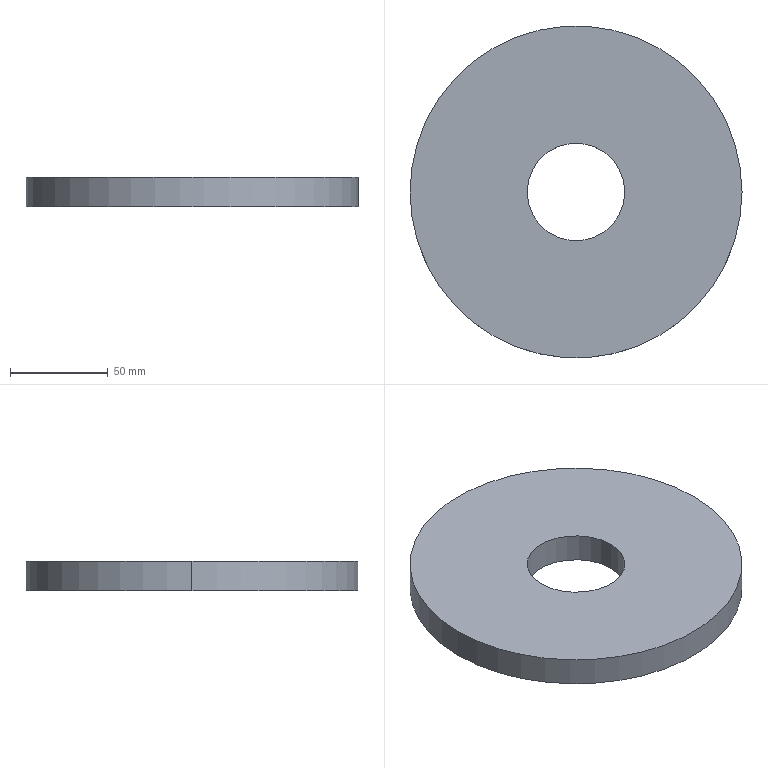Part | SolidWorks | features Extrusion 1 | 1 solid | 6 faces | box 170 x 170 x 15 mm | volume 311018 mm3 | cylinder 4 | plane 2 | commonest cylinder face diameters 50 x2 170 x2
STEP:
#1=CARTESIAN_POINT('',(-25.,0.,15.));
#2=VERTEX_POINT('',#1);
#3=CARTESIAN_POINT('',(25.,0.,15.));
#4=VERTEX_POINT('',#3);
#5=CARTESIAN_POINT('',(0.,0.,15.));
#6=DIRECTION('',(0.,0.,1.));
#7=DIRECTION('',(1.,0.,0.));
#8=AXIS2_PLACEMENT_3D('',#5,#6,#7);
#9=CIRCLE('',#8,25.);
#10=EDGE_CURVE('',#2,#4,#9,.T.);
#11=ORIENTED_EDGE('',*,*,#10,.T.);
#12=CARTESIAN_POINT('',(25.,0.,0.));
#13=VERTEX_POINT('',#12);
#14=CARTESIAN_POINT('',(25.,0.,15.));
#15=DIRECTION('',(0.,0.,-1.));
#16=VECTOR('',#15,1000.);
#17=LINE('',#14,#16);
#18=EDGE_CURVE('',#4,#13,#17,.T.);
#19=ORIENTED_EDGE('',*,*,#18,.T.);
#20=CARTESIAN_POINT('',(-25.,0.,0.));
#21=VERTEX_POINT('',#20);
#22=CARTESIAN_POINT('',(0.,0.,0.));
#23=DIRECTION('',(0.,0.,1.));
#24=DIRECTION('',(1.,0.,0.));
#25=AXIS2_PLACEMENT_3D('',#22,#23,#24);
#26=CIRCLE('',#25,25.);
#27=EDGE_CURVE('',#21,#13,#26,.T.);
#28=ORIENTED_EDGE('',*,*,#27,.F.);
#29=CARTESIAN_POINT('',(-25.,0.,15.));
#30=DIRECTION('',(0.,0.,-1.));
#31=VECTOR('',#30,1000.);
#32=LINE('',#29,#31);
#33=EDGE_CURVE('',#2,#21,#32,.T.);
#34=ORIENTED_EDGE('',*,*,#33,.F.);
#35=EDGE_LOOP('',(#11,#19,#28,#34));
#36=FACE_OUTER_BOUND('',#35,.T.);
#37=CARTESIAN_POINT('',(0.,0.,15.));
#38=DIRECTION('',(0.,0.,-1.));
#39=DIRECTION('',(-1.,0.,0.));
#40=AXIS2_PLACEMENT_3D('',#37,#38,#39);
#41=CYLINDRICAL_SURFACE('',#40,25.);
#42=ADVANCED_FACE('',(#36),#41,.F.);
#43=CARTESIAN_POINT('',(85.,0.,15.));
#44=VERTEX_POINT('',#43);
#45=CARTESIAN_POINT('',(-85.,0.,15.));
#46=VERTEX_POINT('',#45);
#47=CARTESIAN_POINT('',(0.,0.,15.));
#48=DIRECTION('',(0.,0.,1.));
#49=DIRECTION('',(1.,0.,0.));
#50=AXIS2_PLACEMENT_3D('',#47,#48,#49);
#51=CIRCLE('',#50,85.);
#52=EDGE_CURVE('',#44,#46,#51,.T.);
#53=ORIENTED_EDGE('',*,*,#52,.F.);
#54=CARTESIAN_POINT('',(85.,0.,0.));
#55=VERTEX_POINT('',#54);
#56=CARTESIAN_POINT('',(85.,0.,15.));
#57=DIRECTION('',(0.,0.,-1.));
#58=VECTOR('',#57,1000.);
#59=LINE('',#56,#58);
#60=EDGE_CURVE('',#44,#55,#59,.T.);
#61=ORIENTED_EDGE('',*,*,#60,.T.);
#62=CARTESIAN_POINT('',(-85.,0.,0.));
#63=VERTEX_POINT('',#62);
#64=CARTESIAN_POINT('',(0.,0.,0.));
#65=DIRECTION('',(0.,0.,1.));
#66=DIRECTION('',(1.,0.,0.));
#67=AXIS2_PLACEMENT_3D('',#64,#65,#66);
#68=CIRCLE('',#67,85.);
#69=EDGE_CURVE('',#55,#63,#68,.T.);
#70=ORIENTED_EDGE('',*,*,#69,.T.);
#71=CARTESIAN_POINT('',(-85.,0.,15.));
#72=DIRECTION('',(0.,0.,-1.));
#73=VECTOR('',#72,1000.);
#74=LINE('',#71,#73);
#75=EDGE_CURVE('',#46,#63,#74,.T.);
#76=ORIENTED_EDGE('',*,*,#75,.F.);
#77=EDGE_LOOP('',(#53,#61,#70,#76));
#78=FACE_OUTER_BOUND('',#77,.T.);
#79=CARTESIAN_POINT('',(0.,0.,15.));
#80=DIRECTION('',(0.,0.,-1.));
#81=DIRECTION('',(-1.,0.,0.));
#82=AXIS2_PLACEMENT_3D('',#79,#80,#81);
#83=CYLINDRICAL_SURFACE('',#82,85.);
#84=ADVANCED_FACE('',(#78),#83,.T.);
#85=CARTESIAN_POINT('',(0.,0.,15.));
#86=DIRECTION('',(0.,0.,1.));
#87=DIRECTION('',(1.,0.,0.));
#88=AXIS2_PLACEMENT_3D('',#85,#86,#87);
#89=CIRCLE('',#88,85.);
#90=EDGE_CURVE('',#46,#44,#89,.T.);
#91=ORIENTED_EDGE('',*,*,#90,.T.);
#92=ORIENTED_EDGE('',*,*,#52,.T.);
#93=EDGE_LOOP('',(#91,#92));
#94=FACE_OUTER_BOUND('',#93,.T.);
#95=ORIENTED_EDGE('',*,*,#10,.F.);
#96=CARTESIAN_POINT('',(0.,0.,15.));
#97=DIRECTION('',(0.,0.,1.));
#98=DIRECTION('',(1.,0.,0.));
#99=AXIS2_PLACEMENT_3D('',#96,#97,#98);
#100=CIRCLE('',#99,25.);
#101=EDGE_CURVE('',#4,#2,#100,.T.);
#102=ORIENTED_EDGE('',*,*,#101,.F.);
#103=EDGE_LOOP('',(#95,#102));
#104=FACE_BOUND('',#103,.T.);
#105=CARTESIAN_POINT('',(0.,0.,15.));
#106=DIRECTION('',(0.,0.,1.));
#107=DIRECTION('',(1.,0.,0.));
#108=AXIS2_PLACEMENT_3D('',#105,#106,#107);
#109=PLANE('',#108);
#110=ADVANCED_FACE('',(#94,#104),#109,.T.);
#111=CARTESIAN_POINT('',(0.,0.,0.));
#112=DIRECTION('',(0.,0.,1.));
#113=DIRECTION('',(1.,0.,0.));
#114=AXIS2_PLACEMENT_3D('',#111,#112,#113);
#115=CIRCLE('',#114,85.);
#116=EDGE_CURVE('',#63,#55,#115,.T.);
#117=ORIENTED_EDGE('',*,*,#116,.F.);
#118=ORIENTED_EDGE('',*,*,#69,.F.);
#119=EDGE_LOOP('',(#117,#118));
#120=FACE_OUTER_BOUND('',#119,.T.);
#121=ORIENTED_EDGE('',*,*,#27,.T.);
#122=CARTESIAN_POINT('',(0.,0.,0.));
#123=DIRECTION('',(0.,0.,1.));
#124=DIRECTION('',(1.,0.,0.));
#125=AXIS2_PLACEMENT_3D('',#122,#123,#124);
#126=CIRCLE('',#125,25.);
#127=EDGE_CURVE('',#13,#21,#126,.T.);
#128=ORIENTED_EDGE('',*,*,#127,.T.);
#129=EDGE_LOOP('',(#121,#128));
#130=FACE_BOUND('',#129,.T.);
#131=CARTESIAN_POINT('',(0.,0.,0.));
#132=DIRECTION('',(0.,0.,1.));
#133=DIRECTION('',(1.,0.,0.));
#134=AXIS2_PLACEMENT_3D('',#131,#132,#133);
#135=PLANE('',#134);
#136=ADVANCED_FACE('',(#120,#130),#135,.F.);
#137=ORIENTED_EDGE('',*,*,#60,.F.);
#138=ORIENTED_EDGE('',*,*,#90,.F.);
#139=ORIENTED_EDGE('',*,*,#75,.T.);
#140=ORIENTED_EDGE('',*,*,#116,.T.);
#141=EDGE_LOOP('',(#137,#138,#139,#140));
#142=FACE_OUTER_BOUND('',#141,.T.);
#143=CARTESIAN_POINT('',(0.,0.,15.));
#144=DIRECTION('',(0.,0.,-1.));
#145=DIRECTION('',(-1.,0.,0.));
#146=AXIS2_PLACEMENT_3D('',#143,#144,#145);
#147=CYLINDRICAL_SURFACE('',#146,85.);
#148=ADVANCED_FACE('',(#142),#147,.T.);
#149=ORIENTED_EDGE('',*,*,#18,.F.);
#150=ORIENTED_EDGE('',*,*,#101,.T.);
#151=ORIENTED_EDGE('',*,*,#33,.T.);
#152=ORIENTED_EDGE('',*,*,#127,.F.);
#153=EDGE_LOOP('',(#149,#150,#151,#152));
#154=FACE_OUTER_BOUND('',#153,.T.);
#155=CARTESIAN_POINT('',(0.,0.,15.));
#156=DIRECTION('',(0.,0.,-1.));
#157=DIRECTION('',(-1.,0.,0.));
#158=AXIS2_PLACEMENT_3D('',#155,#156,#157);
#159=CYLINDRICAL_SURFACE('',#158,25.);
#160=ADVANCED_FACE('',(#154),#159,.F.);
#161=CLOSED_SHELL('',(#42,#84,#110,#136,#148,#160));
#162=MANIFOLD_SOLID_BREP('',#161);
#163=CARTESIAN_POINT('',(0.,0.,0.));
#164=DIRECTION('',(0.,0.,1.));
#165=DIRECTION('',(1.,0.,0.));
#166=AXIS2_PLACEMENT_3D('',#163,#164,#165);
#167=(LENGTH_UNIT()NAMED_UNIT(*)SI_UNIT(.MILLI.,.METRE.));
#168=UNCERTAINTY_MEASURE_WITH_UNIT(LENGTH_MEASURE(0.00001),#167,'','');
#169=(NAMED_UNIT(*)PLANE_ANGLE_UNIT()SI_UNIT($,.RADIAN.));
#170=(NAMED_UNIT(*)SI_UNIT($,.STERADIAN.)SOLID_ANGLE_UNIT());
#171=(GEOMETRIC_REPRESENTATION_CONTEXT(3)GLOBAL_UNCERTAINTY_ASSIGNED_CONTEXT((#168))GLOBAL_UNIT_ASSIGNED_CONTEXT((#167,#169,#170))REPRESENTATION_CONTEXT('',''));
#172=ADVANCED_BREP_SHAPE_REPRESENTATION('',(#162,#166),#171);